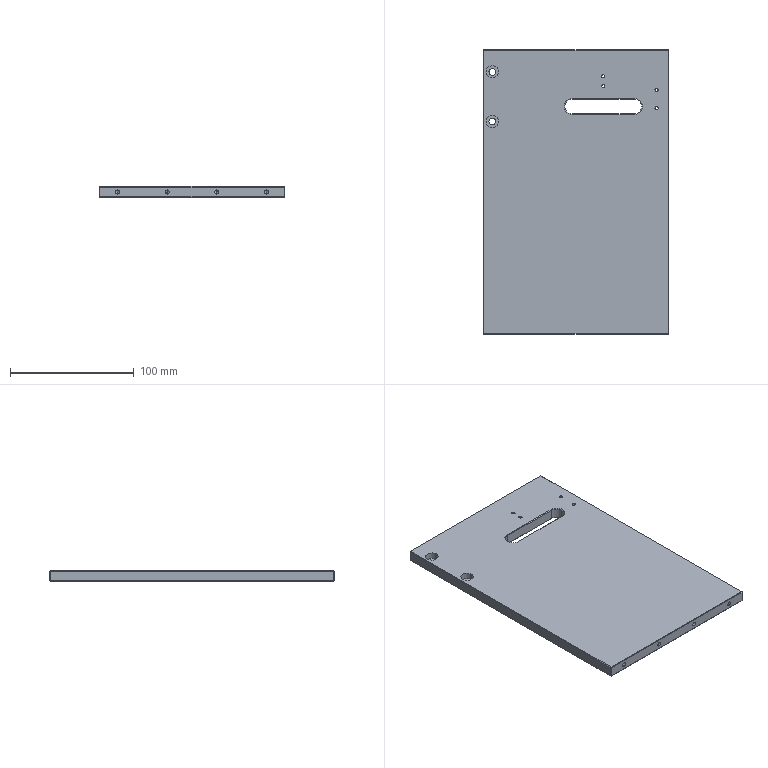Part | STEP file | BPSP-11-001Unloading Support Plate_Default | 1 solid | 108 faces | box 150 x 230 x 9 mm | volume 300493 mm3 | cylinder 41 | plane 41 | cone 26 | commonest cylinder face diameters 3.3 x16 2.5 x12 5.5 x4 10 x4 12 x3 4 x2